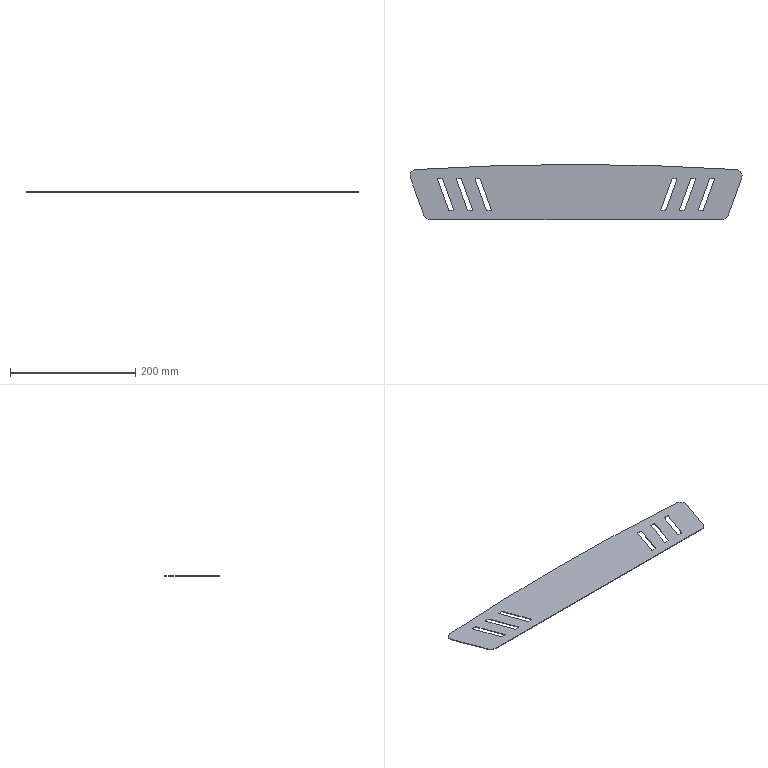Part | STEP file | ZHD 500.75 | 1 solid | 58 faces | box 531.222 x 88.107 x 1 mm | volume 40969 mm3 | cylinder 29 | plane 29 | commonest cylinder face diameters 2 x24 20 x3 20.512 x1 8100 x1